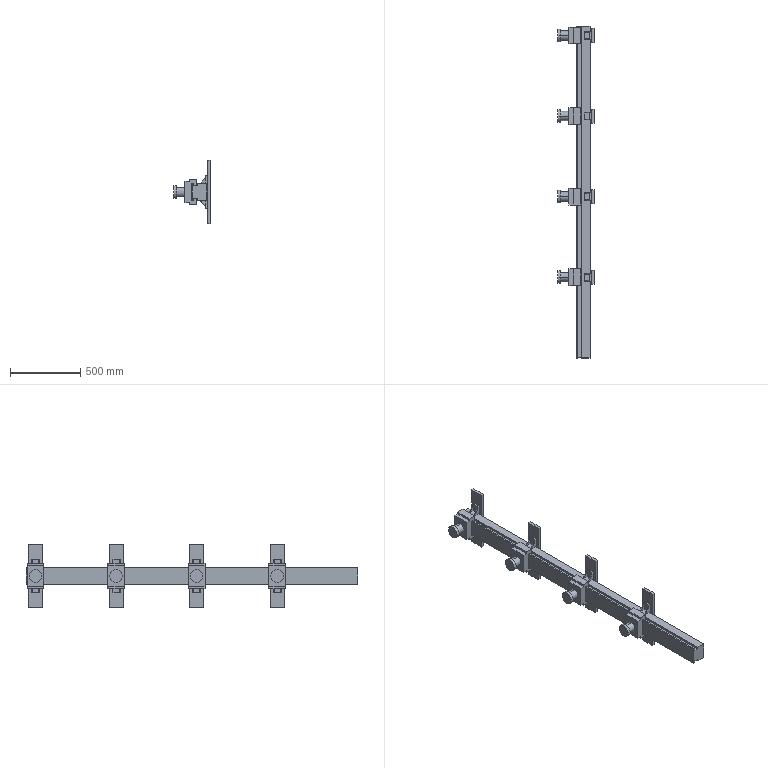Part | SolidWorks | features ICE 9, LPattern 3, Extrusion 1, MirrorPattern 1 | 8 solids | 293 faces | box 260 x 2370 x 450 mm | volume 36834096 mm3 | plane 269 | cylinder 24 | commonest cylinder face diameters 35 x8 67.026 x8 90 x8